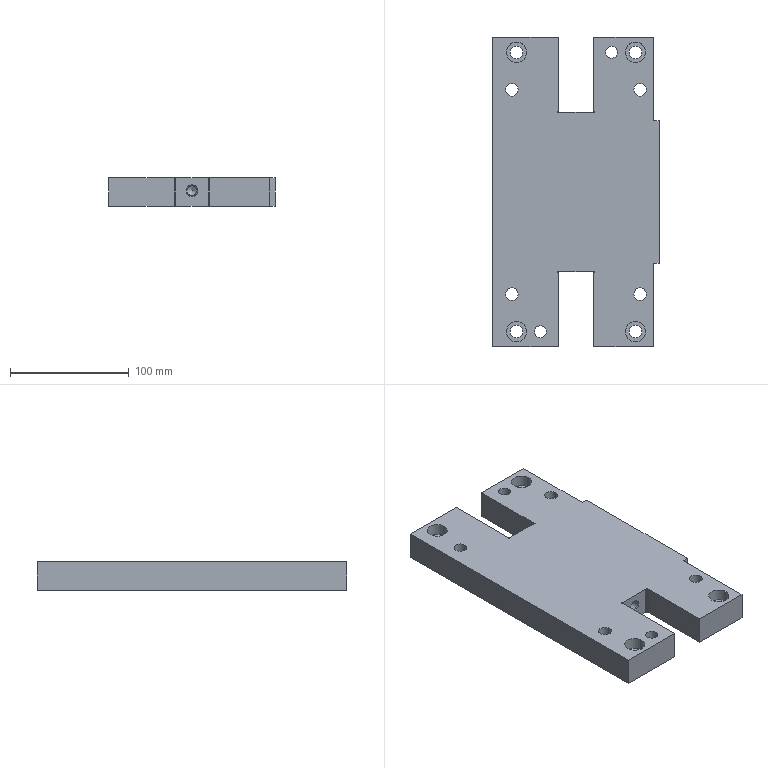Part | STEP file | 冲床-300配套压波_id1034_x_t | 1 solid | 62 faces | box 140 x 260 x 24 mm | volume 727656 mm3 | cylinder 32 | plane 26 | cone 4 | commonest cylinder face diameters 4 x8 10.7 x8 17 x8 1 x4 8.5 x2 10 x2